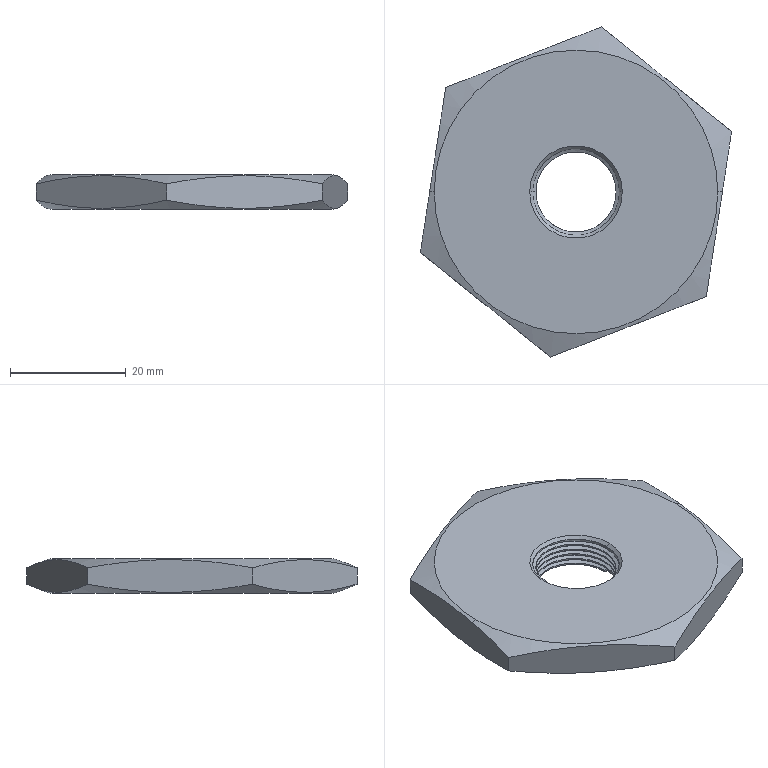Part | STEP file | Lock nut 2 | 1 solid | 33 faces | box 53.803 x 57.066 x 6 mm | volume 11722 mm3 | cylinder 11 | plane 10 | cone 8 | spline 4 | commonest cylinder face diameters 15 x11